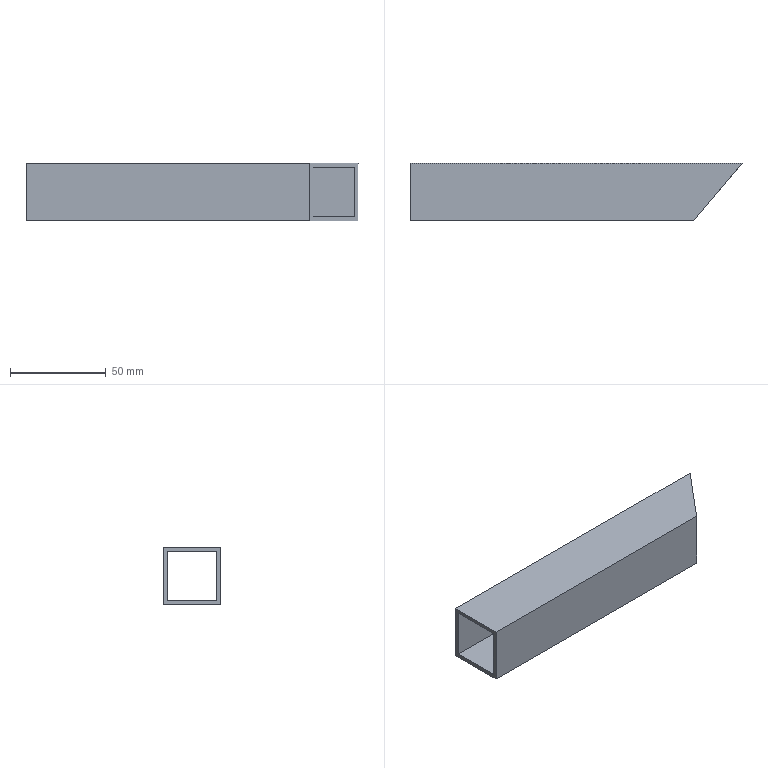Part | NX | features solid 2 | 1 solid | 10 faces | box 173.164 x 30 x 30 mm | volume 35969 mm3 | plane 10
STEP:
#1=CARTESIAN_POINT('',(350.,355.,-75.));
#2=VERTEX_POINT('',#1);
#3=CARTESIAN_POINT('',(350.,325.,-75.));
#4=VERTEX_POINT('',#3);
#5=CARTESIAN_POINT('',(350.,325.,-75.));
#6=DIRECTION('',(0.,-1.,0.));
#7=VECTOR('',#6,1000.);
#8=LINE('',#5,#7);
#9=EDGE_CURVE('',#2,#4,#8,.T.);
#10=ORIENTED_EDGE('',*,*,#9,.F.);
#11=CARTESIAN_POINT('',(523.164,355.,-75.));
#12=VERTEX_POINT('',#11);
#13=CARTESIAN_POINT('',(25.,355.,-75.));
#14=DIRECTION('',(1.,0.,0.));
#15=VECTOR('',#14,1000.);
#16=LINE('',#13,#15);
#17=EDGE_CURVE('',#2,#12,#16,.T.);
#18=ORIENTED_EDGE('',*,*,#17,.T.);
#19=CARTESIAN_POINT('',(497.991,325.,-75.));
#20=VERTEX_POINT('',#19);
#21=CARTESIAN_POINT('',(302.562,92.098,-75.));
#22=DIRECTION('',(0.6428,0.766,0.));
#23=VECTOR('',#22,1000.);
#24=LINE('',#21,#23);
#25=EDGE_CURVE('',#20,#12,#24,.T.);
#26=ORIENTED_EDGE('',*,*,#25,.F.);
#27=CARTESIAN_POINT('',(25.,325.,-75.));
#28=DIRECTION('',(1.,0.,0.));
#29=VECTOR('',#28,1000.);
#30=LINE('',#27,#29);
#31=EDGE_CURVE('',#4,#20,#30,.T.);
#32=ORIENTED_EDGE('',*,*,#31,.F.);
#33=EDGE_LOOP('',(#10,#18,#26,#32));
#34=FACE_BOUND('',#33,.T.);
#35=CARTESIAN_POINT('',(25.,325.,-75.));
#36=DIRECTION('',(0.,0.,1.));
#37=DIRECTION('',(1.,0.,0.));
#38=AXIS2_PLACEMENT_3D('',#35,#36,#37);
#39=PLANE('',#38);
#40=ADVANCED_FACE('',(#34),#39,.F.);
#41=CARTESIAN_POINT('',(350.,355.,-45.));
#42=VERTEX_POINT('',#41);
#43=CARTESIAN_POINT('',(523.164,355.,-45.));
#44=VERTEX_POINT('',#43);
#45=CARTESIAN_POINT('',(25.,355.,-45.));
#46=DIRECTION('',(1.,0.,0.));
#47=VECTOR('',#46,1000.);
#48=LINE('',#45,#47);
#49=EDGE_CURVE('',#42,#44,#48,.T.);
#50=ORIENTED_EDGE('',*,*,#49,.F.);
#51=CARTESIAN_POINT('',(350.,325.,-45.));
#52=VERTEX_POINT('',#51);
#53=CARTESIAN_POINT('',(350.,325.,-45.));
#54=DIRECTION('',(0.,-1.,0.));
#55=VECTOR('',#54,1000.);
#56=LINE('',#53,#55);
#57=EDGE_CURVE('',#42,#52,#56,.T.);
#58=ORIENTED_EDGE('',*,*,#57,.T.);
#59=CARTESIAN_POINT('',(497.991,325.,-45.));
#60=VERTEX_POINT('',#59);
#61=CARTESIAN_POINT('',(25.,325.,-45.));
#62=DIRECTION('',(1.,0.,0.));
#63=VECTOR('',#62,1000.);
#64=LINE('',#61,#63);
#65=EDGE_CURVE('',#52,#60,#64,.T.);
#66=ORIENTED_EDGE('',*,*,#65,.T.);
#67=CARTESIAN_POINT('',(302.562,92.098,-45.));
#68=DIRECTION('',(0.6428,0.766,0.));
#69=VECTOR('',#68,1000.);
#70=LINE('',#67,#69);
#71=EDGE_CURVE('',#60,#44,#70,.T.);
#72=ORIENTED_EDGE('',*,*,#71,.T.);
#73=EDGE_LOOP('',(#50,#58,#66,#72));
#74=FACE_BOUND('',#73,.T.);
#75=CARTESIAN_POINT('',(25.,325.,-45.));
#76=DIRECTION('',(0.,0.,1.));
#77=DIRECTION('',(1.,0.,0.));
#78=AXIS2_PLACEMENT_3D('',#75,#76,#77);
#79=PLANE('',#78);
#80=ADVANCED_FACE('',(#74),#79,.T.);
#81=ORIENTED_EDGE('',*,*,#65,.F.);
#82=CARTESIAN_POINT('',(350.,325.,-75.));
#83=DIRECTION('',(0.,0.,-1.));
#84=VECTOR('',#83,1000.);
#85=LINE('',#82,#84);
#86=EDGE_CURVE('',#52,#4,#85,.T.);
#87=ORIENTED_EDGE('',*,*,#86,.T.);
#88=ORIENTED_EDGE('',*,*,#31,.T.);
#89=CARTESIAN_POINT('',(497.991,325.,-75.));
#90=DIRECTION('',(0.,0.,1.));
#91=VECTOR('',#90,1000.);
#92=LINE('',#89,#91);
#93=EDGE_CURVE('',#20,#60,#92,.T.);
#94=ORIENTED_EDGE('',*,*,#93,.T.);
#95=EDGE_LOOP('',(#81,#87,#88,#94));
#96=FACE_BOUND('',#95,.T.);
#97=CARTESIAN_POINT('',(25.,325.,-75.));
#98=DIRECTION('',(0.,-1.,0.));
#99=DIRECTION('',(1.,0.,0.));
#100=AXIS2_PLACEMENT_3D('',#97,#98,#99);
#101=PLANE('',#100);
#102=ADVANCED_FACE('',(#96),#101,.T.);
#103=ORIENTED_EDGE('',*,*,#17,.F.);
#104=CARTESIAN_POINT('',(350.,355.,-75.));
#105=DIRECTION('',(0.,0.,-1.));
#106=VECTOR('',#105,1000.);
#107=LINE('',#104,#106);
#108=EDGE_CURVE('',#2,#42,#107,.F.);
#109=ORIENTED_EDGE('',*,*,#108,.T.);
#110=ORIENTED_EDGE('',*,*,#49,.T.);
#111=CARTESIAN_POINT('',(523.164,355.,-75.));
#112=DIRECTION('',(0.,0.,-1.));
#113=VECTOR('',#112,1000.);
#114=LINE('',#111,#113);
#115=EDGE_CURVE('',#12,#44,#114,.F.);
#116=ORIENTED_EDGE('',*,*,#115,.F.);
#117=EDGE_LOOP('',(#103,#109,#110,#116));
#118=FACE_BOUND('',#117,.T.);
#119=CARTESIAN_POINT('',(25.,355.,-75.));
#120=DIRECTION('',(0.,-1.,0.));
#121=DIRECTION('',(1.,0.,0.));
#122=AXIS2_PLACEMENT_3D('',#119,#120,#121);
#123=PLANE('',#122);
#124=ADVANCED_FACE('',(#118),#123,.F.);
#125=ORIENTED_EDGE('',*,*,#93,.F.);
#126=ORIENTED_EDGE('',*,*,#25,.T.);
#127=ORIENTED_EDGE('',*,*,#115,.T.);
#128=ORIENTED_EDGE('',*,*,#71,.F.);
#129=EDGE_LOOP('',(#125,#126,#127,#128));
#130=FACE_BOUND('',#129,.T.);
#131=CARTESIAN_POINT('',(499.669,327.,-73.));
#132=VERTEX_POINT('',#131);
#133=CARTESIAN_POINT('',(521.485,353.,-73.));
#134=VERTEX_POINT('',#133);
#135=CARTESIAN_POINT('',(302.562,92.098,-73.));
#136=DIRECTION('',(0.6428,0.766,0.));
#137=VECTOR('',#136,1000.);
#138=LINE('',#135,#137);
#139=EDGE_CURVE('',#132,#134,#138,.T.);
#140=ORIENTED_EDGE('',*,*,#139,.F.);
#141=CARTESIAN_POINT('',(499.669,327.,-47.));
#142=VERTEX_POINT('',#141);
#143=CARTESIAN_POINT('',(499.669,327.,-75.));
#144=DIRECTION('',(0.,0.,1.));
#145=VECTOR('',#144,1000.);
#146=LINE('',#143,#145);
#147=EDGE_CURVE('',#132,#142,#146,.T.);
#148=ORIENTED_EDGE('',*,*,#147,.T.);
#149=CARTESIAN_POINT('',(521.485,353.,-47.));
#150=VERTEX_POINT('',#149);
#151=CARTESIAN_POINT('',(302.562,92.098,-47.));
#152=DIRECTION('',(0.6428,0.766,0.));
#153=VECTOR('',#152,1000.);
#154=LINE('',#151,#153);
#155=EDGE_CURVE('',#142,#150,#154,.T.);
#156=ORIENTED_EDGE('',*,*,#155,.T.);
#157=CARTESIAN_POINT('',(521.485,353.,-75.));
#158=DIRECTION('',(0.,0.,-1.));
#159=VECTOR('',#158,1000.);
#160=LINE('',#157,#159);
#161=EDGE_CURVE('',#134,#150,#160,.F.);
#162=ORIENTED_EDGE('',*,*,#161,.F.);
#163=EDGE_LOOP('',(#140,#148,#156,#162));
#164=FACE_BOUND('',#163,.T.);
#165=CARTESIAN_POINT('',(525.178,357.401,-75.));
#166=DIRECTION('',(0.766,-0.6428,0.));
#167=DIRECTION('',(0.6428,0.766,0.));
#168=AXIS2_PLACEMENT_3D('',#165,#166,#167);
#169=PLANE('',#168);
#170=ADVANCED_FACE('',(#130,#164),#169,.T.);
#171=CARTESIAN_POINT('',(350.,353.,-73.));
#172=VERTEX_POINT('',#171);
#173=CARTESIAN_POINT('',(25.,353.,-73.));
#174=DIRECTION('',(-1.,0.,0.));
#175=VECTOR('',#174,1000.);
#176=LINE('',#173,#175);
#177=EDGE_CURVE('',#172,#134,#176,.F.);
#178=ORIENTED_EDGE('',*,*,#177,.F.);
#179=CARTESIAN_POINT('',(350.,327.,-73.));
#180=VERTEX_POINT('',#179);
#181=CARTESIAN_POINT('',(350.,325.,-73.));
#182=DIRECTION('',(0.,-1.,0.));
#183=VECTOR('',#182,1000.);
#184=LINE('',#181,#183);
#185=EDGE_CURVE('',#172,#180,#184,.T.);
#186=ORIENTED_EDGE('',*,*,#185,.T.);
#187=CARTESIAN_POINT('',(25.,327.,-73.));
#188=DIRECTION('',(1.,0.,0.));
#189=VECTOR('',#188,1000.);
#190=LINE('',#187,#189);
#191=EDGE_CURVE('',#180,#132,#190,.T.);
#192=ORIENTED_EDGE('',*,*,#191,.T.);
#193=ORIENTED_EDGE('',*,*,#139,.T.);
#194=EDGE_LOOP('',(#178,#186,#192,#193));
#195=FACE_BOUND('',#194,.T.);
#196=CARTESIAN_POINT('',(25.,325.,-73.));
#197=DIRECTION('',(0.,0.,1.));
#198=DIRECTION('',(1.,0.,0.));
#199=AXIS2_PLACEMENT_3D('',#196,#197,#198);
#200=PLANE('',#199);
#201=ADVANCED_FACE('',(#195),#200,.T.);
#202=CARTESIAN_POINT('',(350.,353.,-47.));
#203=VERTEX_POINT('',#202);
#204=CARTESIAN_POINT('',(350.,327.,-47.));
#205=VERTEX_POINT('',#204);
#206=CARTESIAN_POINT('',(350.,325.,-47.));
#207=DIRECTION('',(0.,-1.,0.));
#208=VECTOR('',#207,1000.);
#209=LINE('',#206,#208);
#210=EDGE_CURVE('',#203,#205,#209,.T.);
#211=ORIENTED_EDGE('',*,*,#210,.F.);
#212=CARTESIAN_POINT('',(25.,353.,-47.));
#213=DIRECTION('',(-1.,0.,0.));
#214=VECTOR('',#213,1000.);
#215=LINE('',#212,#214);
#216=EDGE_CURVE('',#203,#150,#215,.F.);
#217=ORIENTED_EDGE('',*,*,#216,.T.);
#218=ORIENTED_EDGE('',*,*,#155,.F.);
#219=CARTESIAN_POINT('',(25.,327.,-47.));
#220=DIRECTION('',(1.,0.,0.));
#221=VECTOR('',#220,1000.);
#222=LINE('',#219,#221);
#223=EDGE_CURVE('',#205,#142,#222,.T.);
#224=ORIENTED_EDGE('',*,*,#223,.F.);
#225=EDGE_LOOP('',(#211,#217,#218,#224));
#226=FACE_BOUND('',#225,.T.);
#227=CARTESIAN_POINT('',(25.,325.,-47.));
#228=DIRECTION('',(0.,0.,1.));
#229=DIRECTION('',(1.,0.,0.));
#230=AXIS2_PLACEMENT_3D('',#227,#228,#229);
#231=PLANE('',#230);
#232=ADVANCED_FACE('',(#226),#231,.F.);
#233=CARTESIAN_POINT('',(350.,327.,-75.));
#234=DIRECTION('',(0.,0.,-1.));
#235=VECTOR('',#234,1000.);
#236=LINE('',#233,#235);
#237=EDGE_CURVE('',#205,#180,#236,.T.);
#238=ORIENTED_EDGE('',*,*,#237,.F.);
#239=ORIENTED_EDGE('',*,*,#223,.T.);
#240=ORIENTED_EDGE('',*,*,#147,.F.);
#241=ORIENTED_EDGE('',*,*,#191,.F.);
#242=EDGE_LOOP('',(#238,#239,#240,#241));
#243=FACE_BOUND('',#242,.T.);
#244=CARTESIAN_POINT('',(25.,327.,-75.));
#245=DIRECTION('',(0.,-1.,0.));
#246=DIRECTION('',(1.,0.,0.));
#247=AXIS2_PLACEMENT_3D('',#244,#245,#246);
#248=PLANE('',#247);
#249=ADVANCED_FACE('',(#243),#248,.F.);
#250=CARTESIAN_POINT('',(350.,353.,-75.));
#251=DIRECTION('',(0.,0.,-1.));
#252=VECTOR('',#251,1000.);
#253=LINE('',#250,#252);
#254=EDGE_CURVE('',#172,#203,#253,.F.);
#255=ORIENTED_EDGE('',*,*,#254,.F.);
#256=ORIENTED_EDGE('',*,*,#177,.T.);
#257=ORIENTED_EDGE('',*,*,#161,.T.);
#258=ORIENTED_EDGE('',*,*,#216,.F.);
#259=EDGE_LOOP('',(#255,#256,#257,#258));
#260=FACE_BOUND('',#259,.T.);
#261=CARTESIAN_POINT('',(25.,353.,-75.));
#262=DIRECTION('',(0.,-1.,0.));
#263=DIRECTION('',(1.,0.,0.));
#264=AXIS2_PLACEMENT_3D('',#261,#262,#263);
#265=PLANE('',#264);
#266=ADVANCED_FACE('',(#260),#265,.T.);
#267=ORIENTED_EDGE('',*,*,#57,.F.);
#268=ORIENTED_EDGE('',*,*,#108,.F.);
#269=ORIENTED_EDGE('',*,*,#9,.T.);
#270=ORIENTED_EDGE('',*,*,#86,.F.);
#271=EDGE_LOOP('',(#267,#268,#269,#270));
#272=FACE_BOUND('',#271,.T.);
#273=ORIENTED_EDGE('',*,*,#254,.T.);
#274=ORIENTED_EDGE('',*,*,#210,.T.);
#275=ORIENTED_EDGE('',*,*,#237,.T.);
#276=ORIENTED_EDGE('',*,*,#185,.F.);
#277=EDGE_LOOP('',(#273,#274,#275,#276));
#278=FACE_BOUND('',#277,.T.);
#279=CARTESIAN_POINT('',(350.,360.,-155.));
#280=DIRECTION('',(-1.,0.,0.));
#281=DIRECTION('',(0.,0.,1.));
#282=AXIS2_PLACEMENT_3D('',#279,#280,#281);
#283=PLANE('',#282);
#284=ADVANCED_FACE('',(#272,#278),#283,.T.);
#285=CLOSED_SHELL('',(#40,#80,#102,#124,#170,#201,#232,#249,#266,#284));
#286=MANIFOLD_SOLID_BREP('',#285);
#287=(LENGTH_UNIT()NAMED_UNIT(*)SI_UNIT(.MILLI.,.METRE.));
#288=UNCERTAINTY_MEASURE_WITH_UNIT(LENGTH_MEASURE(0.00001),#287,'','');
#289=(NAMED_UNIT(*)PLANE_ANGLE_UNIT()SI_UNIT($,.RADIAN.));
#290=(NAMED_UNIT(*)SI_UNIT($,.STERADIAN.)SOLID_ANGLE_UNIT());
#291=(GEOMETRIC_REPRESENTATION_CONTEXT(3)GLOBAL_UNCERTAINTY_ASSIGNED_CONTEXT((#288))GLOBAL_UNIT_ASSIGNED_CONTEXT((#287,#289,#290))REPRESENTATION_CONTEXT('',''));
#292=ADVANCED_BREP_SHAPE_REPRESENTATION('',(#286),#291);